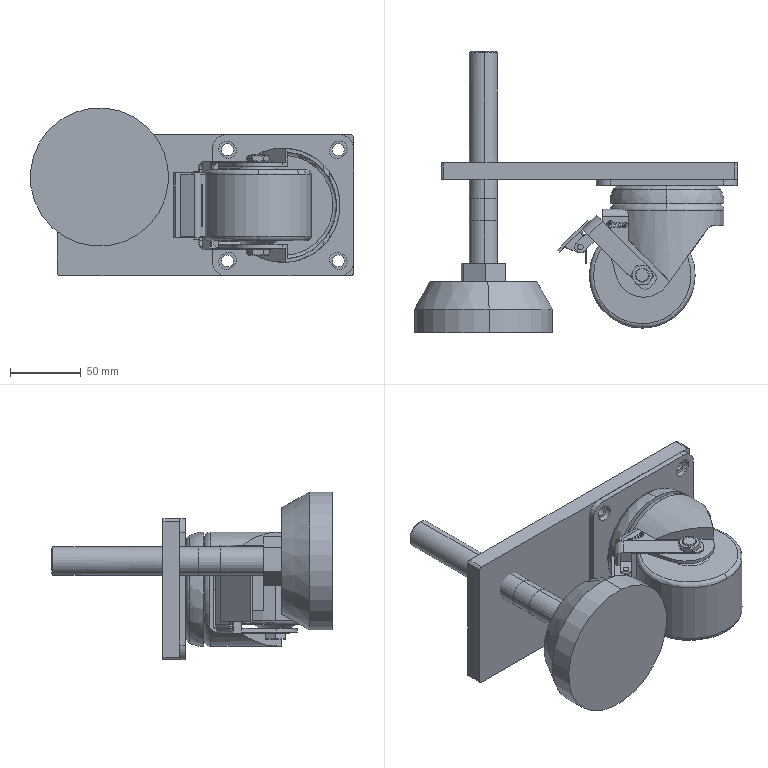Part | SolidWorks | 5 solids | 288 faces | box 229 x 199 x 119 mm | volume 916642 mm3 | plane 150 | cylinder 83 | cone 35 | torus 10 | spline 10 | commonest cylinder face diameters 10 x22 11 x12 4 x10 20 x10 8.5 x8 8 x5